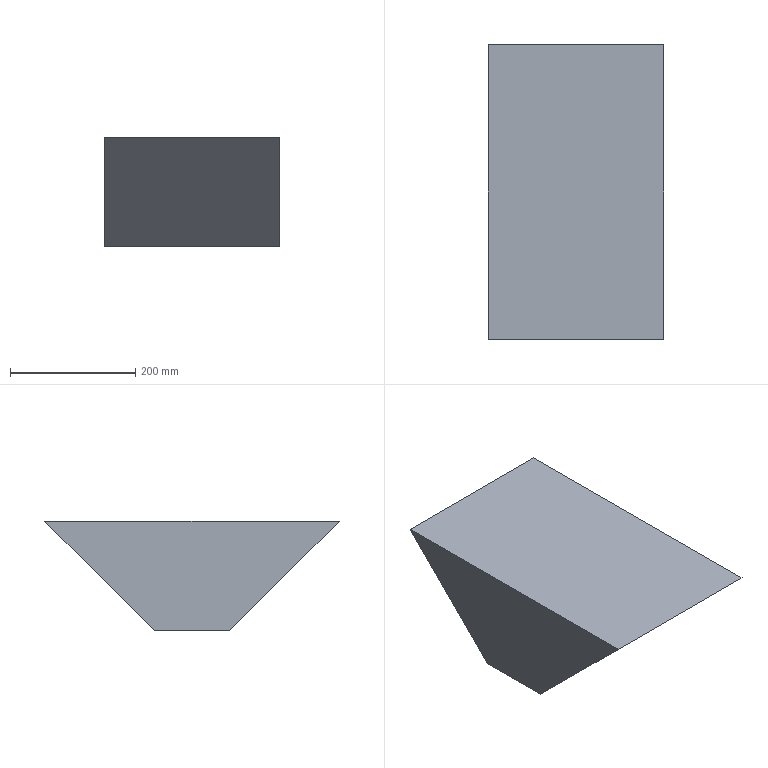Part | NX | features DATUM_CSYS 2, DATUM_PLANE 1, EXTRUDE 1, SKETCH 1 | 1 solid | 6 faces | box 280 x 470 x 175 mm | volume 14455000 mm3 | plane 6
STEP:
#1=CARTESIAN_POINT('',(0.,-235.,175.));
#2=VERTEX_POINT('',#1);
#3=CARTESIAN_POINT('',(0.,-60.,0.));
#4=VERTEX_POINT('',#3);
#5=CARTESIAN_POINT('',(0.,-235.,175.));
#6=DIRECTION('',(0.,0.7071,-0.7071));
#7=VECTOR('',#6,1000.);
#8=LINE('',#5,#7);
#9=EDGE_CURVE('',#2,#4,#8,.T.);
#10=ORIENTED_EDGE('',*,*,#9,.T.);
#11=CARTESIAN_POINT('',(280.,-60.,0.));
#12=VERTEX_POINT('',#11);
#13=CARTESIAN_POINT('',(280.,-60.,0.));
#14=DIRECTION('',(-1.,0.,0.));
#15=VECTOR('',#14,1000.);
#16=LINE('',#13,#15);
#17=EDGE_CURVE('',#12,#4,#16,.T.);
#18=ORIENTED_EDGE('',*,*,#17,.F.);
#19=CARTESIAN_POINT('',(280.,-235.,175.));
#20=VERTEX_POINT('',#19);
#21=CARTESIAN_POINT('',(280.,-235.,175.));
#22=DIRECTION('',(0.,0.7071,-0.7071));
#23=VECTOR('',#22,1000.);
#24=LINE('',#21,#23);
#25=EDGE_CURVE('',#20,#12,#24,.T.);
#26=ORIENTED_EDGE('',*,*,#25,.F.);
#27=CARTESIAN_POINT('',(280.,-235.,175.));
#28=DIRECTION('',(-1.,0.,0.));
#29=VECTOR('',#28,1000.);
#30=LINE('',#27,#29);
#31=EDGE_CURVE('',#20,#2,#30,.T.);
#32=ORIENTED_EDGE('',*,*,#31,.T.);
#33=EDGE_LOOP('',(#10,#18,#26,#32));
#34=FACE_BOUND('',#33,.T.);
#35=CARTESIAN_POINT('',(280.,-235.,175.));
#36=DIRECTION('',(0.,0.7071,0.7071));
#37=DIRECTION('',(0.,-0.7071,0.7071));
#38=AXIS2_PLACEMENT_3D('',#35,#36,#37);
#39=PLANE('',#38);
#40=ADVANCED_FACE('',(#34),#39,.F.);
#41=CARTESIAN_POINT('',(0.,60.,0.));
#42=VERTEX_POINT('',#41);
#43=CARTESIAN_POINT('',(0.,-60.,0.));
#44=DIRECTION('',(0.,1.,0.));
#45=VECTOR('',#44,1000.);
#46=LINE('',#43,#45);
#47=EDGE_CURVE('',#4,#42,#46,.T.);
#48=ORIENTED_EDGE('',*,*,#47,.T.);
#49=CARTESIAN_POINT('',(280.,60.,0.));
#50=VERTEX_POINT('',#49);
#51=CARTESIAN_POINT('',(280.,60.,0.));
#52=DIRECTION('',(-1.,0.,0.));
#53=VECTOR('',#52,1000.);
#54=LINE('',#51,#53);
#55=EDGE_CURVE('',#50,#42,#54,.T.);
#56=ORIENTED_EDGE('',*,*,#55,.F.);
#57=CARTESIAN_POINT('',(280.,-60.,0.));
#58=DIRECTION('',(0.,1.,0.));
#59=VECTOR('',#58,1000.);
#60=LINE('',#57,#59);
#61=EDGE_CURVE('',#12,#50,#60,.T.);
#62=ORIENTED_EDGE('',*,*,#61,.F.);
#63=ORIENTED_EDGE('',*,*,#17,.T.);
#64=EDGE_LOOP('',(#48,#56,#62,#63));
#65=FACE_BOUND('',#64,.T.);
#66=CARTESIAN_POINT('',(280.,-60.,0.));
#67=DIRECTION('',(0.,0.,1.));
#68=DIRECTION('',(1.,0.,0.));
#69=AXIS2_PLACEMENT_3D('',#66,#67,#68);
#70=PLANE('',#69);
#71=ADVANCED_FACE('',(#65),#70,.F.);
#72=CARTESIAN_POINT('',(0.,235.,175.));
#73=VERTEX_POINT('',#72);
#74=CARTESIAN_POINT('',(0.,60.,0.));
#75=DIRECTION('',(0.,0.7071,0.7071));
#76=VECTOR('',#75,1000.);
#77=LINE('',#74,#76);
#78=EDGE_CURVE('',#42,#73,#77,.T.);
#79=ORIENTED_EDGE('',*,*,#78,.T.);
#80=CARTESIAN_POINT('',(280.,235.,175.));
#81=VERTEX_POINT('',#80);
#82=CARTESIAN_POINT('',(280.,235.,175.));
#83=DIRECTION('',(-1.,0.,0.));
#84=VECTOR('',#83,1000.);
#85=LINE('',#82,#84);
#86=EDGE_CURVE('',#81,#73,#85,.T.);
#87=ORIENTED_EDGE('',*,*,#86,.F.);
#88=CARTESIAN_POINT('',(280.,60.,0.));
#89=DIRECTION('',(0.,0.7071,0.7071));
#90=VECTOR('',#89,1000.);
#91=LINE('',#88,#90);
#92=EDGE_CURVE('',#50,#81,#91,.T.);
#93=ORIENTED_EDGE('',*,*,#92,.F.);
#94=ORIENTED_EDGE('',*,*,#55,.T.);
#95=EDGE_LOOP('',(#79,#87,#93,#94));
#96=FACE_BOUND('',#95,.T.);
#97=CARTESIAN_POINT('',(280.,60.,0.));
#98=DIRECTION('',(0.,-0.7071,0.7071));
#99=DIRECTION('',(0.,-0.7071,-0.7071));
#100=AXIS2_PLACEMENT_3D('',#97,#98,#99);
#101=PLANE('',#100);
#102=ADVANCED_FACE('',(#96),#101,.F.);
#103=CARTESIAN_POINT('',(0.,235.,175.));
#104=DIRECTION('',(0.,-1.,0.));
#105=VECTOR('',#104,1000.);
#106=LINE('',#103,#105);
#107=EDGE_CURVE('',#73,#2,#106,.T.);
#108=ORIENTED_EDGE('',*,*,#107,.T.);
#109=ORIENTED_EDGE('',*,*,#31,.F.);
#110=CARTESIAN_POINT('',(280.,235.,175.));
#111=DIRECTION('',(0.,-1.,0.));
#112=VECTOR('',#111,1000.);
#113=LINE('',#110,#112);
#114=EDGE_CURVE('',#81,#20,#113,.T.);
#115=ORIENTED_EDGE('',*,*,#114,.F.);
#116=ORIENTED_EDGE('',*,*,#86,.T.);
#117=EDGE_LOOP('',(#108,#109,#115,#116));
#118=FACE_BOUND('',#117,.T.);
#119=CARTESIAN_POINT('',(280.,235.,175.));
#120=DIRECTION('',(0.,0.,-1.));
#121=DIRECTION('',(-1.,0.,0.));
#122=AXIS2_PLACEMENT_3D('',#119,#120,#121);
#123=PLANE('',#122);
#124=ADVANCED_FACE('',(#118),#123,.F.);
#125=ORIENTED_EDGE('',*,*,#25,.T.);
#126=ORIENTED_EDGE('',*,*,#61,.T.);
#127=ORIENTED_EDGE('',*,*,#92,.T.);
#128=ORIENTED_EDGE('',*,*,#114,.T.);
#129=EDGE_LOOP('',(#125,#126,#127,#128));
#130=FACE_BOUND('',#129,.T.);
#131=CARTESIAN_POINT('',(280.,0.,0.));
#132=DIRECTION('',(1.,0.,0.));
#133=DIRECTION('',(0.,0.,-1.));
#134=AXIS2_PLACEMENT_3D('',#131,#132,#133);
#135=PLANE('',#134);
#136=ADVANCED_FACE('',(#130),#135,.T.);
#137=ORIENTED_EDGE('',*,*,#9,.F.);
#138=ORIENTED_EDGE('',*,*,#107,.F.);
#139=ORIENTED_EDGE('',*,*,#78,.F.);
#140=ORIENTED_EDGE('',*,*,#47,.F.);
#141=EDGE_LOOP('',(#137,#138,#139,#140));
#142=FACE_BOUND('',#141,.T.);
#143=CARTESIAN_POINT('',(0.,0.,0.));
#144=DIRECTION('',(1.,0.,0.));
#145=DIRECTION('',(0.,0.,-1.));
#146=AXIS2_PLACEMENT_3D('',#143,#144,#145);
#147=PLANE('',#146);
#148=ADVANCED_FACE('',(#142),#147,.F.);
#149=CLOSED_SHELL('',(#40,#71,#102,#124,#136,#148));
#150=MANIFOLD_SOLID_BREP('',#149);
#151=(LENGTH_UNIT()NAMED_UNIT(*)SI_UNIT(.MILLI.,.METRE.));
#152=UNCERTAINTY_MEASURE_WITH_UNIT(LENGTH_MEASURE(0.00001),#151,'','');
#153=(NAMED_UNIT(*)PLANE_ANGLE_UNIT()SI_UNIT($,.RADIAN.));
#154=(NAMED_UNIT(*)SI_UNIT($,.STERADIAN.)SOLID_ANGLE_UNIT());
#155=(GEOMETRIC_REPRESENTATION_CONTEXT(3)GLOBAL_UNCERTAINTY_ASSIGNED_CONTEXT((#152))GLOBAL_UNIT_ASSIGNED_CONTEXT((#151,#153,#154))REPRESENTATION_CONTEXT('',''));
#156=ADVANCED_BREP_SHAPE_REPRESENTATION('',(#150),#155);